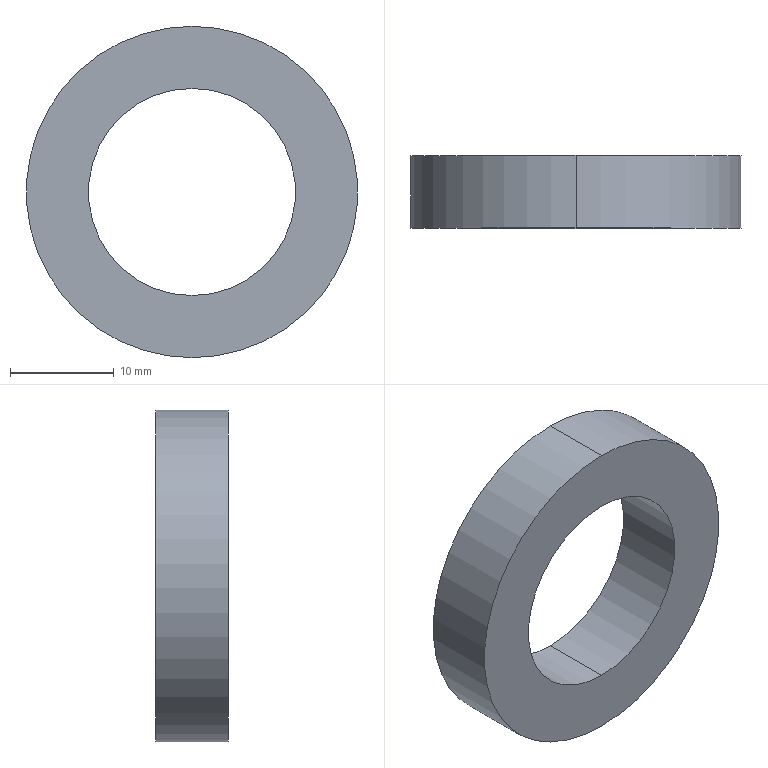Part | STEP file | PN_0087 bearing ZZ6804 | 1 solid | 6 faces | box 32 x 7 x 32 mm | volume 3431 mm3 | cylinder 4 | plane 2 | commonest cylinder face diameters 20 x2 32 x2
STEP:
#1=CARTESIAN_POINT('',(0.,0.,0.));
#2=DIRECTION('',(0.,0.,1.));
#3=DIRECTION('',(1.,0.,0.));
#4=AXIS2_PLACEMENT_3D('',#1,#2,#3);
#5=CARTESIAN_POINT('',(0.,7.,-10.));
#6=VERTEX_POINT('',#5);
#7=CARTESIAN_POINT('',(0.,0.,-10.));
#8=VERTEX_POINT('',#7);
#9=CARTESIAN_POINT('',(0.,7.,-10.));
#10=DIRECTION('',(0.,-1.,0.));
#11=VECTOR('',#10,1.);
#12=LINE('',#9,#11);
#13=CARTESIAN_POINT('',(0.,7.,0.));
#14=DIRECTION('',(0.,-1.,0.));
#15=DIRECTION('',(0.,0.,-1.));
#16=AXIS2_PLACEMENT_3D('',#13,#14,#15);
#17=CYLINDRICAL_SURFACE('',#16,10.);
#18=CARTESIAN_POINT('',(6.283,0.));
#19=DIRECTION('',(0.,1.));
#20=VECTOR('',#19,1.);
#21=LINE('',#18,#20);
#22=(GEOMETRIC_REPRESENTATION_CONTEXT(2)PARAMETRIC_REPRESENTATION_CONTEXT()REPRESENTATION_CONTEXT('',''));
#23=DEFINITIONAL_REPRESENTATION('',(#21),#22);
#24=PCURVE('',#17,#23);
#25=CARTESIAN_POINT('',(0.,7.,0.));
#26=DIRECTION('',(0.,-1.,0.));
#27=DIRECTION('',(0.,0.,-1.));
#28=AXIS2_PLACEMENT_3D('',#25,#26,#27);
#29=CYLINDRICAL_SURFACE('',#28,10.);
#30=CARTESIAN_POINT('',(0.,0.));
#31=DIRECTION('',(0.,1.));
#32=VECTOR('',#31,1.);
#33=LINE('',#30,#32);
#34=(GEOMETRIC_REPRESENTATION_CONTEXT(2)PARAMETRIC_REPRESENTATION_CONTEXT()REPRESENTATION_CONTEXT('',''));
#35=DEFINITIONAL_REPRESENTATION('',(#33),#34);
#36=PCURVE('',#29,#35);
#37=SURFACE_CURVE('',#12,(#24,#36),.PCURVE_S1.);
#38=EDGE_CURVE('',#6,#8,#37,.T.);
#39=ORIENTED_EDGE('',*,*,#38,.T.);
#40=CARTESIAN_POINT('',(0.,0.,10.));
#41=VERTEX_POINT('',#40);
#42=CARTESIAN_POINT('',(0.,0.,0.));
#43=DIRECTION('',(0.,1.,0.));
#44=DIRECTION('',(0.,0.,1.));
#45=AXIS2_PLACEMENT_3D('',#42,#43,#44);
#46=CIRCLE('',#45,10.);
#47=CARTESIAN_POINT('',(9.425,7.));
#48=DIRECTION('',(-1.,0.));
#49=VECTOR('',#48,1.);
#50=LINE('',#47,#49);
#51=(GEOMETRIC_REPRESENTATION_CONTEXT(2)PARAMETRIC_REPRESENTATION_CONTEXT()REPRESENTATION_CONTEXT('',''));
#52=DEFINITIONAL_REPRESENTATION('',(#50),#51);
#53=PCURVE('',#17,#52);
#54=CARTESIAN_POINT('',(0.,0.,0.));
#55=DIRECTION('',(0.,1.,0.));
#56=DIRECTION('',(0.,0.,1.));
#57=AXIS2_PLACEMENT_3D('',#54,#55,#56);
#58=PLANE('',#57);
#59=CARTESIAN_POINT('',(0.,0.));
#60=DIRECTION('',(1.,0.));
#61=AXIS2_PLACEMENT_2D('',#59,#60);
#62=CIRCLE('',#61,10.);
#63=(GEOMETRIC_REPRESENTATION_CONTEXT(2)PARAMETRIC_REPRESENTATION_CONTEXT()REPRESENTATION_CONTEXT('',''));
#64=DEFINITIONAL_REPRESENTATION('',(#62),#63);
#65=PCURVE('',#58,#64);
#66=SURFACE_CURVE('',#46,(#53,#65),.PCURVE_S1.);
#67=EDGE_CURVE('',#8,#41,#66,.T.);
#68=ORIENTED_EDGE('',*,*,#67,.T.);
#69=CARTESIAN_POINT('',(0.,7.,10.));
#70=VERTEX_POINT('',#69);
#71=CARTESIAN_POINT('',(0.,7.,10.));
#72=DIRECTION('',(0.,-1.,0.));
#73=VECTOR('',#72,1.);
#74=LINE('',#71,#73);
#75=CARTESIAN_POINT('',(3.142,0.));
#76=DIRECTION('',(0.,1.));
#77=VECTOR('',#76,1.);
#78=LINE('',#75,#77);
#79=(GEOMETRIC_REPRESENTATION_CONTEXT(2)PARAMETRIC_REPRESENTATION_CONTEXT()REPRESENTATION_CONTEXT('',''));
#80=DEFINITIONAL_REPRESENTATION('',(#78),#79);
#81=PCURVE('',#17,#80);
#82=CARTESIAN_POINT('',(3.142,0.));
#83=DIRECTION('',(0.,1.));
#84=VECTOR('',#83,1.);
#85=LINE('',#82,#84);
#86=(GEOMETRIC_REPRESENTATION_CONTEXT(2)PARAMETRIC_REPRESENTATION_CONTEXT()REPRESENTATION_CONTEXT('',''));
#87=DEFINITIONAL_REPRESENTATION('',(#85),#86);
#88=PCURVE('',#29,#87);
#89=SURFACE_CURVE('',#74,(#81,#88),.PCURVE_S1.);
#90=EDGE_CURVE('',#70,#41,#89,.T.);
#91=ORIENTED_EDGE('',*,*,#90,.F.);
#92=CARTESIAN_POINT('',(0.,7.,0.));
#93=DIRECTION('',(0.,1.,0.));
#94=DIRECTION('',(0.,0.,1.));
#95=AXIS2_PLACEMENT_3D('',#92,#93,#94);
#96=CIRCLE('',#95,10.);
#97=CARTESIAN_POINT('',(9.425,0.));
#98=DIRECTION('',(-1.,0.));
#99=VECTOR('',#98,1.);
#100=LINE('',#97,#99);
#101=(GEOMETRIC_REPRESENTATION_CONTEXT(2)PARAMETRIC_REPRESENTATION_CONTEXT()REPRESENTATION_CONTEXT('',''));
#102=DEFINITIONAL_REPRESENTATION('',(#100),#101);
#103=PCURVE('',#17,#102);
#104=CARTESIAN_POINT('',(0.,7.,0.));
#105=DIRECTION('',(0.,1.,0.));
#106=DIRECTION('',(0.,0.,1.));
#107=AXIS2_PLACEMENT_3D('',#104,#105,#106);
#108=PLANE('',#107);
#109=CARTESIAN_POINT('',(0.,0.));
#110=DIRECTION('',(1.,0.));
#111=AXIS2_PLACEMENT_2D('',#109,#110);
#112=CIRCLE('',#111,10.);
#113=(GEOMETRIC_REPRESENTATION_CONTEXT(2)PARAMETRIC_REPRESENTATION_CONTEXT()REPRESENTATION_CONTEXT('',''));
#114=DEFINITIONAL_REPRESENTATION('',(#112),#113);
#115=PCURVE('',#108,#114);
#116=SURFACE_CURVE('',#96,(#103,#115),.PCURVE_S1.);
#117=EDGE_CURVE('',#6,#70,#116,.T.);
#118=ORIENTED_EDGE('',*,*,#117,.F.);
#119=EDGE_LOOP('',(#39,#68,#91,#118));
#120=FACE_BOUND('',#119,.F.);
#121=ADVANCED_FACE('',(#120),#17,.F.);
#122=CARTESIAN_POINT('',(0.,7.,16.));
#123=VERTEX_POINT('',#122);
#124=CARTESIAN_POINT('',(0.,7.,-16.));
#125=VERTEX_POINT('',#124);
#126=CARTESIAN_POINT('',(0.,7.,0.));
#127=DIRECTION('',(0.,1.,0.));
#128=DIRECTION('',(0.,0.,1.));
#129=AXIS2_PLACEMENT_3D('',#126,#127,#128);
#130=CIRCLE('',#129,16.);
#131=CARTESIAN_POINT('',(0.,7.,0.));
#132=DIRECTION('',(0.,-1.,0.));
#133=DIRECTION('',(0.,0.,-1.));
#134=AXIS2_PLACEMENT_3D('',#131,#132,#133);
#135=CYLINDRICAL_SURFACE('',#134,16.);
#136=CARTESIAN_POINT('',(3.142,0.));
#137=DIRECTION('',(-1.,0.));
#138=VECTOR('',#137,1.);
#139=LINE('',#136,#138);
#140=(GEOMETRIC_REPRESENTATION_CONTEXT(2)PARAMETRIC_REPRESENTATION_CONTEXT()REPRESENTATION_CONTEXT('',''));
#141=DEFINITIONAL_REPRESENTATION('',(#139),#140);
#142=PCURVE('',#135,#141);
#143=CARTESIAN_POINT('',(0.,0.));
#144=DIRECTION('',(1.,0.));
#145=AXIS2_PLACEMENT_2D('',#143,#144);
#146=CIRCLE('',#145,16.);
#147=(GEOMETRIC_REPRESENTATION_CONTEXT(2)PARAMETRIC_REPRESENTATION_CONTEXT()REPRESENTATION_CONTEXT('',''));
#148=DEFINITIONAL_REPRESENTATION('',(#146),#147);
#149=PCURVE('',#108,#148);
#150=SURFACE_CURVE('',#130,(#142,#149),.PCURVE_S1.);
#151=EDGE_CURVE('',#123,#125,#150,.T.);
#152=ORIENTED_EDGE('',*,*,#151,.F.);
#153=CARTESIAN_POINT('',(0.,0.,16.));
#154=VERTEX_POINT('',#153);
#155=CARTESIAN_POINT('',(0.,7.,16.));
#156=DIRECTION('',(0.,-1.,0.));
#157=VECTOR('',#156,1.);
#158=LINE('',#155,#157);
#159=CARTESIAN_POINT('',(3.142,0.));
#160=DIRECTION('',(0.,1.));
#161=VECTOR('',#160,1.);
#162=LINE('',#159,#161);
#163=(GEOMETRIC_REPRESENTATION_CONTEXT(2)PARAMETRIC_REPRESENTATION_CONTEXT()REPRESENTATION_CONTEXT('',''));
#164=DEFINITIONAL_REPRESENTATION('',(#162),#163);
#165=PCURVE('',#135,#164);
#166=CARTESIAN_POINT('',(0.,7.,0.));
#167=DIRECTION('',(0.,-1.,0.));
#168=DIRECTION('',(0.,0.,-1.));
#169=AXIS2_PLACEMENT_3D('',#166,#167,#168);
#170=CYLINDRICAL_SURFACE('',#169,16.);
#171=CARTESIAN_POINT('',(3.142,0.));
#172=DIRECTION('',(0.,1.));
#173=VECTOR('',#172,1.);
#174=LINE('',#171,#173);
#175=(GEOMETRIC_REPRESENTATION_CONTEXT(2)PARAMETRIC_REPRESENTATION_CONTEXT()REPRESENTATION_CONTEXT('',''));
#176=DEFINITIONAL_REPRESENTATION('',(#174),#175);
#177=PCURVE('',#170,#176);
#178=SURFACE_CURVE('',#158,(#165,#177),.PCURVE_S1.);
#179=EDGE_CURVE('',#123,#154,#178,.T.);
#180=ORIENTED_EDGE('',*,*,#179,.T.);
#181=CARTESIAN_POINT('',(0.,0.,-16.));
#182=VERTEX_POINT('',#181);
#183=CARTESIAN_POINT('',(0.,0.,0.));
#184=DIRECTION('',(0.,1.,0.));
#185=DIRECTION('',(0.,0.,1.));
#186=AXIS2_PLACEMENT_3D('',#183,#184,#185);
#187=CIRCLE('',#186,16.);
#188=CARTESIAN_POINT('',(3.142,7.));
#189=DIRECTION('',(-1.,0.));
#190=VECTOR('',#189,1.);
#191=LINE('',#188,#190);
#192=(GEOMETRIC_REPRESENTATION_CONTEXT(2)PARAMETRIC_REPRESENTATION_CONTEXT()REPRESENTATION_CONTEXT('',''));
#193=DEFINITIONAL_REPRESENTATION('',(#191),#192);
#194=PCURVE('',#135,#193);
#195=CARTESIAN_POINT('',(0.,0.));
#196=DIRECTION('',(1.,0.));
#197=AXIS2_PLACEMENT_2D('',#195,#196);
#198=CIRCLE('',#197,16.);
#199=(GEOMETRIC_REPRESENTATION_CONTEXT(2)PARAMETRIC_REPRESENTATION_CONTEXT()REPRESENTATION_CONTEXT('',''));
#200=DEFINITIONAL_REPRESENTATION('',(#198),#199);
#201=PCURVE('',#58,#200);
#202=SURFACE_CURVE('',#187,(#194,#201),.PCURVE_S1.);
#203=EDGE_CURVE('',#154,#182,#202,.T.);
#204=ORIENTED_EDGE('',*,*,#203,.T.);
#205=CARTESIAN_POINT('',(0.,7.,-16.));
#206=DIRECTION('',(0.,-1.,0.));
#207=VECTOR('',#206,1.);
#208=LINE('',#205,#207);
#209=CARTESIAN_POINT('',(0.,0.));
#210=DIRECTION('',(0.,1.));
#211=VECTOR('',#210,1.);
#212=LINE('',#209,#211);
#213=(GEOMETRIC_REPRESENTATION_CONTEXT(2)PARAMETRIC_REPRESENTATION_CONTEXT()REPRESENTATION_CONTEXT('',''));
#214=DEFINITIONAL_REPRESENTATION('',(#212),#213);
#215=PCURVE('',#135,#214);
#216=CARTESIAN_POINT('',(6.283,0.));
#217=DIRECTION('',(0.,1.));
#218=VECTOR('',#217,1.);
#219=LINE('',#216,#218);
#220=(GEOMETRIC_REPRESENTATION_CONTEXT(2)PARAMETRIC_REPRESENTATION_CONTEXT()REPRESENTATION_CONTEXT('',''));
#221=DEFINITIONAL_REPRESENTATION('',(#219),#220);
#222=PCURVE('',#170,#221);
#223=SURFACE_CURVE('',#208,(#215,#222),.PCURVE_S1.);
#224=EDGE_CURVE('',#125,#182,#223,.T.);
#225=ORIENTED_EDGE('',*,*,#224,.F.);
#226=EDGE_LOOP('',(#152,#180,#204,#225));
#227=FACE_BOUND('',#226,.T.);
#228=ADVANCED_FACE('',(#227),#135,.T.);
#229=CARTESIAN_POINT('',(0.,7.,0.));
#230=DIRECTION('',(0.,1.,0.));
#231=DIRECTION('',(0.,0.,1.));
#232=AXIS2_PLACEMENT_3D('',#229,#230,#231);
#233=CIRCLE('',#232,16.);
#234=CARTESIAN_POINT('',(0.,0.));
#235=DIRECTION('',(1.,0.));
#236=AXIS2_PLACEMENT_2D('',#234,#235);
#237=CIRCLE('',#236,16.);
#238=(GEOMETRIC_REPRESENTATION_CONTEXT(2)PARAMETRIC_REPRESENTATION_CONTEXT()REPRESENTATION_CONTEXT('',''));
#239=DEFINITIONAL_REPRESENTATION('',(#237),#238);
#240=PCURVE('',#108,#239);
#241=CARTESIAN_POINT('',(9.425,0.));
#242=DIRECTION('',(-1.,0.));
#243=VECTOR('',#242,1.);
#244=LINE('',#241,#243);
#245=(GEOMETRIC_REPRESENTATION_CONTEXT(2)PARAMETRIC_REPRESENTATION_CONTEXT()REPRESENTATION_CONTEXT('',''));
#246=DEFINITIONAL_REPRESENTATION('',(#244),#245);
#247=PCURVE('',#170,#246);
#248=SURFACE_CURVE('',#233,(#240,#247),.PCURVE_S1.);
#249=EDGE_CURVE('',#125,#123,#248,.T.);
#250=ORIENTED_EDGE('',*,*,#249,.T.);
#251=ORIENTED_EDGE('',*,*,#151,.T.);
#252=EDGE_LOOP('',(#250,#251));
#253=FACE_BOUND('',#252,.T.);
#254=ORIENTED_EDGE('',*,*,#117,.F.);
#255=CARTESIAN_POINT('',(0.,7.,0.));
#256=DIRECTION('',(0.,1.,0.));
#257=DIRECTION('',(0.,0.,1.));
#258=AXIS2_PLACEMENT_3D('',#255,#256,#257);
#259=CIRCLE('',#258,10.);
#260=CARTESIAN_POINT('',(0.,0.));
#261=DIRECTION('',(1.,0.));
#262=AXIS2_PLACEMENT_2D('',#260,#261);
#263=CIRCLE('',#262,10.);
#264=(GEOMETRIC_REPRESENTATION_CONTEXT(2)PARAMETRIC_REPRESENTATION_CONTEXT()REPRESENTATION_CONTEXT('',''));
#265=DEFINITIONAL_REPRESENTATION('',(#263),#264);
#266=PCURVE('',#108,#265);
#267=CARTESIAN_POINT('',(3.142,0.));
#268=DIRECTION('',(-1.,0.));
#269=VECTOR('',#268,1.);
#270=LINE('',#267,#269);
#271=(GEOMETRIC_REPRESENTATION_CONTEXT(2)PARAMETRIC_REPRESENTATION_CONTEXT()REPRESENTATION_CONTEXT('',''));
#272=DEFINITIONAL_REPRESENTATION('',(#270),#271);
#273=PCURVE('',#29,#272);
#274=SURFACE_CURVE('',#259,(#266,#273),.PCURVE_S1.);
#275=EDGE_CURVE('',#70,#6,#274,.T.);
#276=ORIENTED_EDGE('',*,*,#275,.F.);
#277=EDGE_LOOP('',(#254,#276));
#278=FACE_BOUND('',#277,.T.);
#279=ADVANCED_FACE('',(#253,#278),#108,.T.);
#280=CARTESIAN_POINT('',(0.,0.,0.));
#281=DIRECTION('',(0.,1.,0.));
#282=DIRECTION('',(0.,0.,1.));
#283=AXIS2_PLACEMENT_3D('',#280,#281,#282);
#284=CIRCLE('',#283,16.);
#285=CARTESIAN_POINT('',(0.,0.));
#286=DIRECTION('',(1.,0.));
#287=AXIS2_PLACEMENT_2D('',#285,#286);
#288=CIRCLE('',#287,16.);
#289=(GEOMETRIC_REPRESENTATION_CONTEXT(2)PARAMETRIC_REPRESENTATION_CONTEXT()REPRESENTATION_CONTEXT('',''));
#290=DEFINITIONAL_REPRESENTATION('',(#288),#289);
#291=PCURVE('',#58,#290);
#292=CARTESIAN_POINT('',(9.425,7.));
#293=DIRECTION('',(-1.,0.));
#294=VECTOR('',#293,1.);
#295=LINE('',#292,#294);
#296=(GEOMETRIC_REPRESENTATION_CONTEXT(2)PARAMETRIC_REPRESENTATION_CONTEXT()REPRESENTATION_CONTEXT('',''));
#297=DEFINITIONAL_REPRESENTATION('',(#295),#296);
#298=PCURVE('',#170,#297);
#299=SURFACE_CURVE('',#284,(#291,#298),.PCURVE_S1.);
#300=EDGE_CURVE('',#182,#154,#299,.T.);
#301=ORIENTED_EDGE('',*,*,#300,.F.);
#302=ORIENTED_EDGE('',*,*,#203,.F.);
#303=EDGE_LOOP('',(#301,#302));
#304=FACE_BOUND('',#303,.T.);
#305=ORIENTED_EDGE('',*,*,#67,.T.);
#306=CARTESIAN_POINT('',(0.,0.,0.));
#307=DIRECTION('',(0.,1.,0.));
#308=DIRECTION('',(0.,0.,1.));
#309=AXIS2_PLACEMENT_3D('',#306,#307,#308);
#310=CIRCLE('',#309,10.);
#311=CARTESIAN_POINT('',(0.,0.));
#312=DIRECTION('',(1.,0.));
#313=AXIS2_PLACEMENT_2D('',#311,#312);
#314=CIRCLE('',#313,10.);
#315=(GEOMETRIC_REPRESENTATION_CONTEXT(2)PARAMETRIC_REPRESENTATION_CONTEXT()REPRESENTATION_CONTEXT('',''));
#316=DEFINITIONAL_REPRESENTATION('',(#314),#315);
#317=PCURVE('',#58,#316);
#318=CARTESIAN_POINT('',(3.142,7.));
#319=DIRECTION('',(-1.,0.));
#320=VECTOR('',#319,1.);
#321=LINE('',#318,#320);
#322=(GEOMETRIC_REPRESENTATION_CONTEXT(2)PARAMETRIC_REPRESENTATION_CONTEXT()REPRESENTATION_CONTEXT('',''));
#323=DEFINITIONAL_REPRESENTATION('',(#321),#322);
#324=PCURVE('',#29,#323);
#325=SURFACE_CURVE('',#310,(#317,#324),.PCURVE_S1.);
#326=EDGE_CURVE('',#41,#8,#325,.T.);
#327=ORIENTED_EDGE('',*,*,#326,.T.);
#328=EDGE_LOOP('',(#305,#327));
#329=FACE_BOUND('',#328,.T.);
#330=ADVANCED_FACE('',(#304,#329),#58,.F.);
#331=ORIENTED_EDGE('',*,*,#179,.F.);
#332=ORIENTED_EDGE('',*,*,#249,.F.);
#333=ORIENTED_EDGE('',*,*,#224,.T.);
#334=ORIENTED_EDGE('',*,*,#300,.T.);
#335=EDGE_LOOP('',(#331,#332,#333,#334));
#336=FACE_BOUND('',#335,.T.);
#337=ADVANCED_FACE('',(#336),#170,.T.);
#338=ORIENTED_EDGE('',*,*,#326,.T.);
#339=ORIENTED_EDGE('',*,*,#38,.F.);
#340=ORIENTED_EDGE('',*,*,#275,.F.);
#341=ORIENTED_EDGE('',*,*,#90,.T.);
#342=EDGE_LOOP('',(#338,#339,#340,#341));
#343=FACE_BOUND('',#342,.F.);
#344=ADVANCED_FACE('',(#343),#29,.F.);
#345=CLOSED_SHELL('',(#121,#228,#279,#330,#337,#344));
#346=MANIFOLD_SOLID_BREP('',#345);
#347=(LENGTH_UNIT()NAMED_UNIT(*)SI_UNIT(.MILLI.,.METRE.));
#348=UNCERTAINTY_MEASURE_WITH_UNIT(LENGTH_MEASURE(0.0000001),#347,'','');
#349=(NAMED_UNIT(*)PLANE_ANGLE_UNIT()SI_UNIT($,.RADIAN.));
#350=(NAMED_UNIT(*)SI_UNIT($,.STERADIAN.)SOLID_ANGLE_UNIT());
#351=(GEOMETRIC_REPRESENTATION_CONTEXT(3)GLOBAL_UNCERTAINTY_ASSIGNED_CONTEXT((#348))GLOBAL_UNIT_ASSIGNED_CONTEXT((#347,#349,#350))REPRESENTATION_CONTEXT('',''));
#352=ADVANCED_BREP_SHAPE_REPRESENTATION('',(#4,#346),#351);